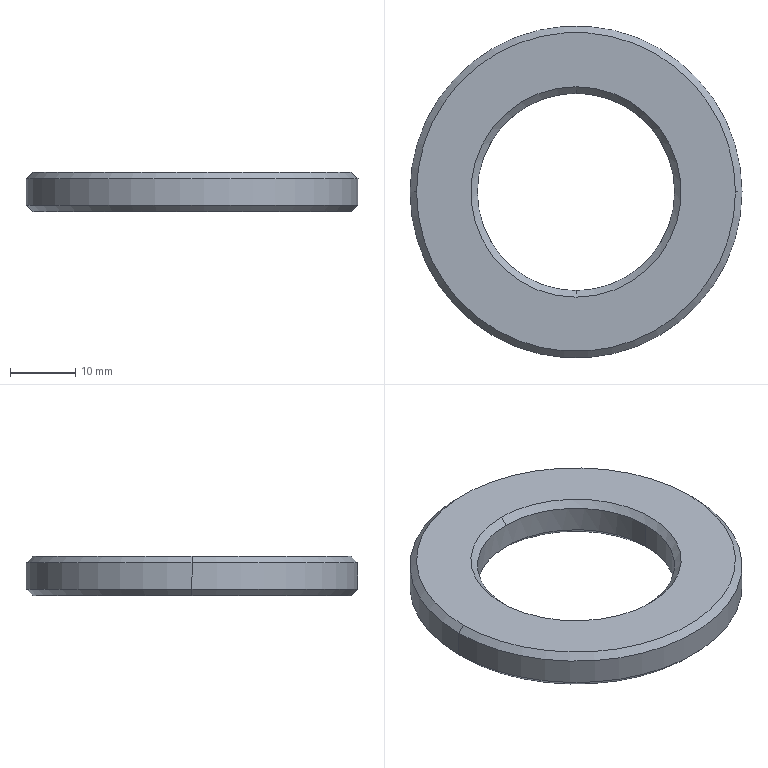Part | SolidWorks | features BaseBody 1 | 1 solid | 14 faces | box 50.8 x 50.8 x 6 mm | volume 7609 mm3 | cone 8 | cylinder 4 | plane 2 | commonest cylinder face diameters 30.2 x2 50.8 x2
STEP:
#1=CARTESIAN_POINT('',(14.226,0.1942,1.));
#2=VERTEX_POINT('',#1);
#3=CARTESIAN_POINT('',(-15.974,0.1942,1.));
#4=VERTEX_POINT('',#3);
#5=CARTESIAN_POINT('',(-0.8738,0.1942,1.));
#6=DIRECTION('',(0.,0.,-1.));
#7=DIRECTION('',(-1.,0.,0.));
#8=AXIS2_PLACEMENT_3D('',#5,#6,#7);
#9=CIRCLE('',#8,15.1);
#10=EDGE_CURVE('',#2,#4,#9,.T.);
#11=ORIENTED_EDGE('',*,*,#10,.F.);
#12=CARTESIAN_POINT('',(15.226,0.1942,0.));
#13=VERTEX_POINT('',#12);
#14=CARTESIAN_POINT('',(15.226,0.1942,0.));
#15=DIRECTION('',(0.7071,0.,-0.7071));
#16=VECTOR('',#15,1000.);
#17=LINE('',#14,#16);
#18=EDGE_CURVE('',#2,#13,#17,.T.);
#19=ORIENTED_EDGE('',*,*,#18,.T.);
#20=CARTESIAN_POINT('',(-16.974,0.1942,0.));
#21=VERTEX_POINT('',#20);
#22=CARTESIAN_POINT('',(-0.8738,0.1942,0.));
#23=DIRECTION('',(0.,0.,1.));
#24=DIRECTION('',(-1.,0.,0.));
#25=AXIS2_PLACEMENT_3D('',#22,#23,#24);
#26=CIRCLE('',#25,16.1);
#27=EDGE_CURVE('',#21,#13,#26,.T.);
#28=ORIENTED_EDGE('',*,*,#27,.F.);
#29=CARTESIAN_POINT('',(-16.974,0.1942,0.));
#30=DIRECTION('',(-0.7071,0.,-0.7071));
#31=VECTOR('',#30,1000.);
#32=LINE('',#29,#31);
#33=EDGE_CURVE('',#4,#21,#32,.T.);
#34=ORIENTED_EDGE('',*,*,#33,.F.);
#35=EDGE_LOOP('',(#11,#19,#28,#34));
#36=FACE_OUTER_BOUND('',#35,.T.);
#37=CARTESIAN_POINT('',(-0.8738,0.1942,0.));
#38=DIRECTION('',(0.,0.,-1.));
#39=DIRECTION('',(-1.,0.,0.));
#40=AXIS2_PLACEMENT_3D('',#37,#38,#39);
#41=CONICAL_SURFACE('',#40,16.1,0.7854);
#42=ADVANCED_FACE('',(#36),#41,.F.);
#43=CARTESIAN_POINT('',(-25.274,0.1942,0.));
#44=VERTEX_POINT('',#43);
#45=CARTESIAN_POINT('',(23.526,0.1942,0.));
#46=VERTEX_POINT('',#45);
#47=CARTESIAN_POINT('',(-0.8738,0.1942,0.));
#48=DIRECTION('',(0.,0.,-1.));
#49=DIRECTION('',(1.,0.,0.));
#50=AXIS2_PLACEMENT_3D('',#47,#48,#49);
#51=CIRCLE('',#50,24.4);
#52=EDGE_CURVE('',#44,#46,#51,.T.);
#53=ORIENTED_EDGE('',*,*,#52,.F.);
#54=CARTESIAN_POINT('',(-26.274,0.1942,1.));
#55=VERTEX_POINT('',#54);
#56=CARTESIAN_POINT('',(-26.274,0.1942,1.));
#57=DIRECTION('',(-0.7071,0.,0.7071));
#58=VECTOR('',#57,1000.);
#59=LINE('',#56,#58);
#60=EDGE_CURVE('',#44,#55,#59,.T.);
#61=ORIENTED_EDGE('',*,*,#60,.T.);
#62=CARTESIAN_POINT('',(24.526,0.1942,1.));
#63=VERTEX_POINT('',#62);
#64=CARTESIAN_POINT('',(-0.8738,0.1942,1.));
#65=DIRECTION('',(0.,0.,-1.));
#66=DIRECTION('',(-1.,0.,0.));
#67=AXIS2_PLACEMENT_3D('',#64,#65,#66);
#68=CIRCLE('',#67,25.4);
#69=EDGE_CURVE('',#55,#63,#68,.T.);
#70=ORIENTED_EDGE('',*,*,#69,.T.);
#71=CARTESIAN_POINT('',(24.526,0.1942,1.));
#72=DIRECTION('',(0.7071,0.,0.7071));
#73=VECTOR('',#72,1000.);
#74=LINE('',#71,#73);
#75=EDGE_CURVE('',#46,#63,#74,.T.);
#76=ORIENTED_EDGE('',*,*,#75,.F.);
#77=EDGE_LOOP('',(#53,#61,#70,#76));
#78=FACE_OUTER_BOUND('',#77,.T.);
#79=CARTESIAN_POINT('',(-0.8738,0.1942,1.));
#80=DIRECTION('',(0.,0.,1.));
#81=DIRECTION('',(1.,0.,0.));
#82=AXIS2_PLACEMENT_3D('',#79,#80,#81);
#83=CONICAL_SURFACE('',#82,25.4,0.7854);
#84=ADVANCED_FACE('',(#78),#83,.T.);
#85=ORIENTED_EDGE('',*,*,#10,.T.);
#86=CARTESIAN_POINT('',(-15.974,0.1942,5.));
#87=VERTEX_POINT('',#86);
#88=CARTESIAN_POINT('',(-15.974,0.1942,0.));
#89=DIRECTION('',(0.,0.,1.));
#90=VECTOR('',#89,1000.);
#91=LINE('',#88,#90);
#92=EDGE_CURVE('',#4,#87,#91,.T.);
#93=ORIENTED_EDGE('',*,*,#92,.T.);
#94=CARTESIAN_POINT('',(-0.8738,-14.906,5.));
#95=VERTEX_POINT('',#94);
#96=CARTESIAN_POINT('',(-0.8738,0.1942,5.));
#97=DIRECTION('',(0.,0.,-1.));
#98=DIRECTION('',(1.,0.,0.));
#99=AXIS2_PLACEMENT_3D('',#96,#97,#98);
#100=CIRCLE('',#99,15.1);
#101=EDGE_CURVE('',#95,#87,#100,.T.);
#102=ORIENTED_EDGE('',*,*,#101,.F.);
#103=CARTESIAN_POINT('',(14.226,0.1942,5.));
#104=VERTEX_POINT('',#103);
#105=CARTESIAN_POINT('',(-0.8738,0.1942,5.));
#106=DIRECTION('',(0.,0.,-1.));
#107=DIRECTION('',(1.,0.,0.));
#108=AXIS2_PLACEMENT_3D('',#105,#106,#107);
#109=CIRCLE('',#108,15.1);
#110=EDGE_CURVE('',#104,#95,#109,.T.);
#111=ORIENTED_EDGE('',*,*,#110,.F.);
#112=CARTESIAN_POINT('',(14.226,0.1942,0.));
#113=DIRECTION('',(0.,0.,1.));
#114=VECTOR('',#113,1000.);
#115=LINE('',#112,#114);
#116=EDGE_CURVE('',#2,#104,#115,.T.);
#117=ORIENTED_EDGE('',*,*,#116,.F.);
#118=EDGE_LOOP('',(#85,#93,#102,#111,#117));
#119=FACE_OUTER_BOUND('',#118,.T.);
#120=CARTESIAN_POINT('',(-0.8738,0.1942,0.));
#121=DIRECTION('',(0.,0.,1.));
#122=DIRECTION('',(1.,0.,0.));
#123=AXIS2_PLACEMENT_3D('',#120,#121,#122);
#124=CYLINDRICAL_SURFACE('',#123,15.1);
#125=ADVANCED_FACE('',(#119),#124,.F.);
#126=ORIENTED_EDGE('',*,*,#69,.F.);
#127=CARTESIAN_POINT('',(-26.274,0.1942,5.));
#128=VERTEX_POINT('',#127);
#129=CARTESIAN_POINT('',(-26.274,0.1942,0.));
#130=DIRECTION('',(0.,0.,1.));
#131=VECTOR('',#130,1000.);
#132=LINE('',#129,#131);
#133=EDGE_CURVE('',#55,#128,#132,.T.);
#134=ORIENTED_EDGE('',*,*,#133,.T.);
#135=CARTESIAN_POINT('',(24.526,0.1942,5.));
#136=VERTEX_POINT('',#135);
#137=CARTESIAN_POINT('',(-0.8738,0.1942,5.));
#138=DIRECTION('',(0.,0.,-1.));
#139=DIRECTION('',(1.,0.,0.));
#140=AXIS2_PLACEMENT_3D('',#137,#138,#139);
#141=CIRCLE('',#140,25.4);
#142=EDGE_CURVE('',#128,#136,#141,.T.);
#143=ORIENTED_EDGE('',*,*,#142,.T.);
#144=CARTESIAN_POINT('',(24.526,0.1942,0.));
#145=DIRECTION('',(0.,0.,1.));
#146=VECTOR('',#145,1000.);
#147=LINE('',#144,#146);
#148=EDGE_CURVE('',#63,#136,#147,.T.);
#149=ORIENTED_EDGE('',*,*,#148,.F.);
#150=EDGE_LOOP('',(#126,#134,#143,#149));
#151=FACE_OUTER_BOUND('',#150,.T.);
#152=CARTESIAN_POINT('',(-0.8738,0.1942,0.));
#153=DIRECTION('',(0.,0.,1.));
#154=DIRECTION('',(1.,0.,0.));
#155=AXIS2_PLACEMENT_3D('',#152,#153,#154);
#156=CYLINDRICAL_SURFACE('',#155,25.4);
#157=ADVANCED_FACE('',(#151),#156,.T.);
#158=ORIENTED_EDGE('',*,*,#101,.T.);
#159=CARTESIAN_POINT('',(-0.8738,15.294,5.));
#160=VERTEX_POINT('',#159);
#161=CARTESIAN_POINT('',(-0.8738,0.1942,5.));
#162=DIRECTION('',(0.,0.,-1.));
#163=DIRECTION('',(1.,0.,0.));
#164=AXIS2_PLACEMENT_3D('',#161,#162,#163);
#165=CIRCLE('',#164,15.1);
#166=EDGE_CURVE('',#87,#160,#165,.T.);
#167=ORIENTED_EDGE('',*,*,#166,.T.);
#168=CARTESIAN_POINT('',(-0.8738,16.294,6.));
#169=VERTEX_POINT('',#168);
#170=CARTESIAN_POINT('',(-0.8738,16.294,6.));
#171=DIRECTION('',(0.,0.7071,0.7071));
#172=VECTOR('',#171,1000.);
#173=LINE('',#170,#172);
#174=EDGE_CURVE('',#160,#169,#173,.T.);
#175=ORIENTED_EDGE('',*,*,#174,.T.);
#176=CARTESIAN_POINT('',(-0.8738,-15.906,6.));
#177=VERTEX_POINT('',#176);
#178=CARTESIAN_POINT('',(-0.8738,0.1942,6.));
#179=DIRECTION('',(0.,0.,-1.));
#180=DIRECTION('',(0.,-1.,0.));
#181=AXIS2_PLACEMENT_3D('',#178,#179,#180);
#182=CIRCLE('',#181,16.1);
#183=EDGE_CURVE('',#177,#169,#182,.T.);
#184=ORIENTED_EDGE('',*,*,#183,.F.);
#185=CARTESIAN_POINT('',(-0.8738,-15.906,6.));
#186=DIRECTION('',(0.,-0.7071,0.7071));
#187=VECTOR('',#186,1000.);
#188=LINE('',#185,#187);
#189=EDGE_CURVE('',#95,#177,#188,.T.);
#190=ORIENTED_EDGE('',*,*,#189,.F.);
#191=EDGE_LOOP('',(#158,#167,#175,#184,#190));
#192=FACE_OUTER_BOUND('',#191,.T.);
#193=CARTESIAN_POINT('',(-0.8738,0.1942,6.));
#194=DIRECTION('',(0.,0.,1.));
#195=DIRECTION('',(0.,-1.,0.));
#196=AXIS2_PLACEMENT_3D('',#193,#194,#195);
#197=CONICAL_SURFACE('',#196,16.1,0.7854);
#198=ADVANCED_FACE('',(#192),#197,.F.);
#199=CARTESIAN_POINT('',(-25.274,0.1942,6.));
#200=VERTEX_POINT('',#199);
#201=CARTESIAN_POINT('',(23.526,0.1942,6.));
#202=VERTEX_POINT('',#201);
#203=CARTESIAN_POINT('',(-0.8738,0.1942,6.));
#204=DIRECTION('',(0.,0.,-1.));
#205=DIRECTION('',(-1.,0.,0.));
#206=AXIS2_PLACEMENT_3D('',#203,#204,#205);
#207=CIRCLE('',#206,24.4);
#208=EDGE_CURVE('',#200,#202,#207,.T.);
#209=ORIENTED_EDGE('',*,*,#208,.T.);
#210=CARTESIAN_POINT('',(24.526,0.1942,5.));
#211=DIRECTION('',(0.7071,0.,-0.7071));
#212=VECTOR('',#211,1000.);
#213=LINE('',#210,#212);
#214=EDGE_CURVE('',#202,#136,#213,.T.);
#215=ORIENTED_EDGE('',*,*,#214,.T.);
#216=ORIENTED_EDGE('',*,*,#142,.F.);
#217=CARTESIAN_POINT('',(-26.274,0.1942,5.));
#218=DIRECTION('',(-0.7071,0.,-0.7071));
#219=VECTOR('',#218,1000.);
#220=LINE('',#217,#219);
#221=EDGE_CURVE('',#200,#128,#220,.T.);
#222=ORIENTED_EDGE('',*,*,#221,.F.);
#223=EDGE_LOOP('',(#209,#215,#216,#222));
#224=FACE_OUTER_BOUND('',#223,.T.);
#225=CARTESIAN_POINT('',(-0.8738,0.1942,5.));
#226=DIRECTION('',(0.,0.,-1.));
#227=DIRECTION('',(-1.,0.,0.));
#228=AXIS2_PLACEMENT_3D('',#225,#226,#227);
#229=CONICAL_SURFACE('',#228,25.4,0.7854);
#230=ADVANCED_FACE('',(#224),#229,.T.);
#231=ORIENTED_EDGE('',*,*,#27,.T.);
#232=CARTESIAN_POINT('',(-0.8738,0.1942,0.));
#233=DIRECTION('',(0.,0.,1.));
#234=DIRECTION('',(-1.,0.,0.));
#235=AXIS2_PLACEMENT_3D('',#232,#233,#234);
#236=CIRCLE('',#235,16.1);
#237=EDGE_CURVE('',#13,#21,#236,.T.);
#238=ORIENTED_EDGE('',*,*,#237,.T.);
#239=EDGE_LOOP('',(#231,#238));
#240=FACE_BOUND('',#239,.T.);
#241=CARTESIAN_POINT('',(-0.8738,0.1942,0.));
#242=DIRECTION('',(0.,0.,-1.));
#243=DIRECTION('',(1.,0.,0.));
#244=AXIS2_PLACEMENT_3D('',#241,#242,#243);
#245=CIRCLE('',#244,24.4);
#246=EDGE_CURVE('',#46,#44,#245,.T.);
#247=ORIENTED_EDGE('',*,*,#246,.T.);
#248=ORIENTED_EDGE('',*,*,#52,.T.);
#249=EDGE_LOOP('',(#247,#248));
#250=FACE_OUTER_BOUND('',#249,.T.);
#251=CARTESIAN_POINT('',(-0.8738,0.1942,0.));
#252=DIRECTION('',(0.,0.,-1.));
#253=DIRECTION('',(-1.,0.,0.));
#254=AXIS2_PLACEMENT_3D('',#251,#252,#253);
#255=PLANE('',#254);
#256=ADVANCED_FACE('',(#240,#250),#255,.T.);
#257=ORIENTED_EDGE('',*,*,#18,.F.);
#258=CARTESIAN_POINT('',(-0.8738,0.1942,1.));
#259=DIRECTION('',(0.,0.,-1.));
#260=DIRECTION('',(-1.,0.,0.));
#261=AXIS2_PLACEMENT_3D('',#258,#259,#260);
#262=CIRCLE('',#261,15.1);
#263=EDGE_CURVE('',#4,#2,#262,.T.);
#264=ORIENTED_EDGE('',*,*,#263,.F.);
#265=ORIENTED_EDGE('',*,*,#33,.T.);
#266=ORIENTED_EDGE('',*,*,#237,.F.);
#267=EDGE_LOOP('',(#257,#264,#265,#266));
#268=FACE_OUTER_BOUND('',#267,.T.);
#269=CARTESIAN_POINT('',(-0.8738,0.1942,0.));
#270=DIRECTION('',(0.,0.,-1.));
#271=DIRECTION('',(-1.,0.,0.));
#272=AXIS2_PLACEMENT_3D('',#269,#270,#271);
#273=CONICAL_SURFACE('',#272,16.1,0.7854);
#274=ADVANCED_FACE('',(#268),#273,.F.);
#275=ORIENTED_EDGE('',*,*,#60,.F.);
#276=ORIENTED_EDGE('',*,*,#246,.F.);
#277=ORIENTED_EDGE('',*,*,#75,.T.);
#278=CARTESIAN_POINT('',(-0.8738,0.1942,1.));
#279=DIRECTION('',(0.,0.,-1.));
#280=DIRECTION('',(-1.,0.,0.));
#281=AXIS2_PLACEMENT_3D('',#278,#279,#280);
#282=CIRCLE('',#281,25.4);
#283=EDGE_CURVE('',#63,#55,#282,.T.);
#284=ORIENTED_EDGE('',*,*,#283,.T.);
#285=EDGE_LOOP('',(#275,#276,#277,#284));
#286=FACE_OUTER_BOUND('',#285,.T.);
#287=CARTESIAN_POINT('',(-0.8738,0.1942,1.));
#288=DIRECTION('',(0.,0.,1.));
#289=DIRECTION('',(1.,0.,0.));
#290=AXIS2_PLACEMENT_3D('',#287,#288,#289);
#291=CONICAL_SURFACE('',#290,25.4,0.7854);
#292=ADVANCED_FACE('',(#286),#291,.T.);
#293=ORIENTED_EDGE('',*,*,#92,.F.);
#294=ORIENTED_EDGE('',*,*,#263,.T.);
#295=ORIENTED_EDGE('',*,*,#116,.T.);
#296=CARTESIAN_POINT('',(-0.8738,0.1942,5.));
#297=DIRECTION('',(0.,0.,-1.));
#298=DIRECTION('',(1.,0.,0.));
#299=AXIS2_PLACEMENT_3D('',#296,#297,#298);
#300=CIRCLE('',#299,15.1);
#301=EDGE_CURVE('',#160,#104,#300,.T.);
#302=ORIENTED_EDGE('',*,*,#301,.F.);
#303=ORIENTED_EDGE('',*,*,#166,.F.);
#304=EDGE_LOOP('',(#293,#294,#295,#302,#303));
#305=FACE_OUTER_BOUND('',#304,.T.);
#306=CARTESIAN_POINT('',(-0.8738,0.1942,0.));
#307=DIRECTION('',(0.,0.,1.));
#308=DIRECTION('',(1.,0.,0.));
#309=AXIS2_PLACEMENT_3D('',#306,#307,#308);
#310=CYLINDRICAL_SURFACE('',#309,15.1);
#311=ADVANCED_FACE('',(#305),#310,.F.);
#312=ORIENTED_EDGE('',*,*,#133,.F.);
#313=ORIENTED_EDGE('',*,*,#283,.F.);
#314=ORIENTED_EDGE('',*,*,#148,.T.);
#315=CARTESIAN_POINT('',(-0.8738,0.1942,5.));
#316=DIRECTION('',(0.,0.,-1.));
#317=DIRECTION('',(1.,0.,0.));
#318=AXIS2_PLACEMENT_3D('',#315,#316,#317);
#319=CIRCLE('',#318,25.4);
#320=EDGE_CURVE('',#136,#128,#319,.T.);
#321=ORIENTED_EDGE('',*,*,#320,.T.);
#322=EDGE_LOOP('',(#312,#313,#314,#321));
#323=FACE_OUTER_BOUND('',#322,.T.);
#324=CARTESIAN_POINT('',(-0.8738,0.1942,0.));
#325=DIRECTION('',(0.,0.,1.));
#326=DIRECTION('',(1.,0.,0.));
#327=AXIS2_PLACEMENT_3D('',#324,#325,#326);
#328=CYLINDRICAL_SURFACE('',#327,25.4);
#329=ADVANCED_FACE('',(#323),#328,.T.);
#330=ORIENTED_EDGE('',*,*,#174,.F.);
#331=ORIENTED_EDGE('',*,*,#301,.T.);
#332=ORIENTED_EDGE('',*,*,#110,.T.);
#333=ORIENTED_EDGE('',*,*,#189,.T.);
#334=CARTESIAN_POINT('',(-0.8738,0.1942,6.));
#335=DIRECTION('',(0.,0.,-1.));
#336=DIRECTION('',(0.,-1.,0.));
#337=AXIS2_PLACEMENT_3D('',#334,#335,#336);
#338=CIRCLE('',#337,16.1);
#339=EDGE_CURVE('',#169,#177,#338,.T.);
#340=ORIENTED_EDGE('',*,*,#339,.F.);
#341=EDGE_LOOP('',(#330,#331,#332,#333,#340));
#342=FACE_OUTER_BOUND('',#341,.T.);
#343=CARTESIAN_POINT('',(-0.8738,0.1942,6.));
#344=DIRECTION('',(0.,0.,1.));
#345=DIRECTION('',(0.,-1.,0.));
#346=AXIS2_PLACEMENT_3D('',#343,#344,#345);
#347=CONICAL_SURFACE('',#346,16.1,0.7854);
#348=ADVANCED_FACE('',(#342),#347,.F.);
#349=ORIENTED_EDGE('',*,*,#214,.F.);
#350=CARTESIAN_POINT('',(-0.8738,0.1942,6.));
#351=DIRECTION('',(0.,0.,-1.));
#352=DIRECTION('',(-1.,0.,0.));
#353=AXIS2_PLACEMENT_3D('',#350,#351,#352);
#354=CIRCLE('',#353,24.4);
#355=EDGE_CURVE('',#202,#200,#354,.T.);
#356=ORIENTED_EDGE('',*,*,#355,.T.);
#357=ORIENTED_EDGE('',*,*,#221,.T.);
#358=ORIENTED_EDGE('',*,*,#320,.F.);
#359=EDGE_LOOP('',(#349,#356,#357,#358));
#360=FACE_OUTER_BOUND('',#359,.T.);
#361=CARTESIAN_POINT('',(-0.8738,0.1942,5.));
#362=DIRECTION('',(0.,0.,-1.));
#363=DIRECTION('',(-1.,0.,0.));
#364=AXIS2_PLACEMENT_3D('',#361,#362,#363);
#365=CONICAL_SURFACE('',#364,25.4,0.7854);
#366=ADVANCED_FACE('',(#360),#365,.T.);
#367=ORIENTED_EDGE('',*,*,#183,.T.);
#368=ORIENTED_EDGE('',*,*,#339,.T.);
#369=EDGE_LOOP('',(#367,#368));
#370=FACE_BOUND('',#369,.T.);
#371=ORIENTED_EDGE('',*,*,#208,.F.);
#372=ORIENTED_EDGE('',*,*,#355,.F.);
#373=EDGE_LOOP('',(#371,#372));
#374=FACE_OUTER_BOUND('',#373,.T.);
#375=CARTESIAN_POINT('',(-0.8738,0.1942,6.));
#376=DIRECTION('',(0.,0.,-1.));
#377=DIRECTION('',(-1.,0.,0.));
#378=AXIS2_PLACEMENT_3D('',#375,#376,#377);
#379=PLANE('',#378);
#380=ADVANCED_FACE('',(#370,#374),#379,.F.);
#381=CLOSED_SHELL('',(#42,#84,#125,#157,#198,#230,#256,#274,#292,#311,#329,#348,#366,#380));
#382=MANIFOLD_SOLID_BREP('',#381);
#383=CARTESIAN_POINT('',(0.,0.,0.));
#384=DIRECTION('',(0.,0.,1.));
#385=DIRECTION('',(1.,0.,0.));
#386=AXIS2_PLACEMENT_3D('',#383,#384,#385);
#387=(LENGTH_UNIT()NAMED_UNIT(*)SI_UNIT(.MILLI.,.METRE.));
#388=UNCERTAINTY_MEASURE_WITH_UNIT(LENGTH_MEASURE(0.00001),#387,'','');
#389=(NAMED_UNIT(*)PLANE_ANGLE_UNIT()SI_UNIT($,.RADIAN.));
#390=(NAMED_UNIT(*)SI_UNIT($,.STERADIAN.)SOLID_ANGLE_UNIT());
#391=(GEOMETRIC_REPRESENTATION_CONTEXT(3)GLOBAL_UNCERTAINTY_ASSIGNED_CONTEXT((#388))GLOBAL_UNIT_ASSIGNED_CONTEXT((#387,#389,#390))REPRESENTATION_CONTEXT('',''));
#392=ADVANCED_BREP_SHAPE_REPRESENTATION('',(#382,#386),#391);